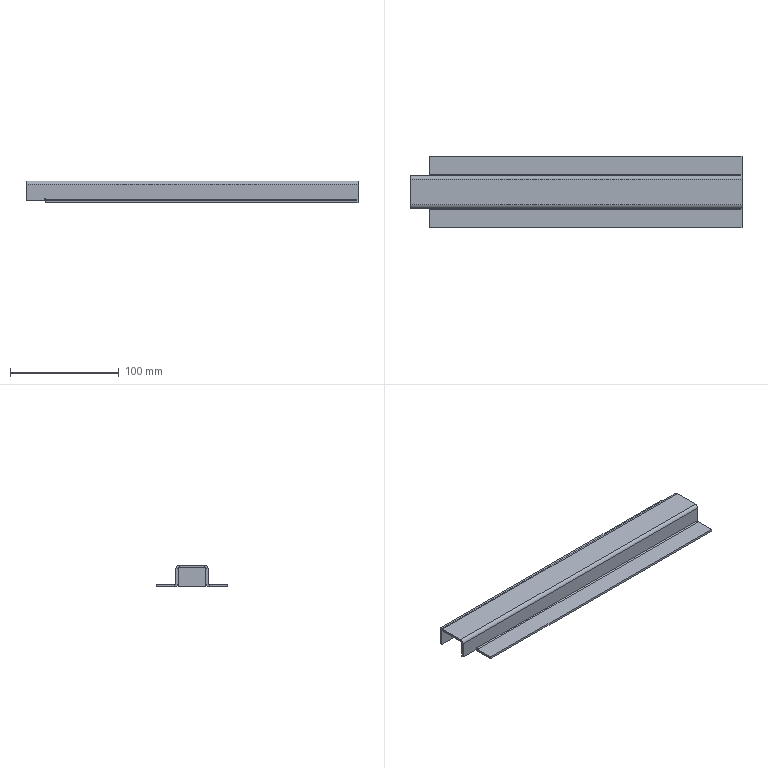Part | SolidWorks | features BaseBody 2 | 2 solids | 54 faces | box 304.9 x 65.5 x 20 mm | volume 59332 mm3 | plane 44 | cylinder 10 | commonest cylinder face diameters 2 x6 6 x4
STEP:
#1=CARTESIAN_POINT('',(-152.45,-14.75,-18.));
#2=VERTEX_POINT('',#1);
#3=CARTESIAN_POINT('',(-152.45,-12.75,-18.));
#4=VERTEX_POINT('',#3);
#5=CARTESIAN_POINT('',(-152.45,-32.75,-18.));
#6=DIRECTION('',(0.,1.,0.));
#7=VECTOR('',#6,1000.);
#8=LINE('',#5,#7);
#9=EDGE_CURVE('',#2,#4,#8,.T.);
#10=ORIENTED_EDGE('',*,*,#9,.T.);
#11=CARTESIAN_POINT('',(-135.45,-12.75,-18.));
#12=VERTEX_POINT('',#11);
#13=CARTESIAN_POINT('',(0.,-12.75,-18.));
#14=DIRECTION('',(1.,0.,0.));
#15=VECTOR('',#14,1000.);
#16=LINE('',#13,#15);
#17=EDGE_CURVE('',#4,#12,#16,.T.);
#18=ORIENTED_EDGE('',*,*,#17,.T.);
#19=CARTESIAN_POINT('',(-135.45,-14.75,-18.));
#20=VERTEX_POINT('',#19);
#21=CARTESIAN_POINT('',(-135.45,-32.75,-18.));
#22=DIRECTION('',(0.,1.,0.));
#23=VECTOR('',#22,1000.);
#24=LINE('',#21,#23);
#25=EDGE_CURVE('',#20,#12,#24,.T.);
#26=ORIENTED_EDGE('',*,*,#25,.F.);
#27=CARTESIAN_POINT('',(0.,-14.75,-18.));
#28=DIRECTION('',(1.,0.,0.));
#29=VECTOR('',#28,1000.);
#30=LINE('',#27,#29);
#31=EDGE_CURVE('',#2,#20,#30,.T.);
#32=ORIENTED_EDGE('',*,*,#31,.F.);
#33=EDGE_LOOP('',(#10,#18,#26,#32));
#34=FACE_OUTER_BOUND('',#33,.T.);
#35=CARTESIAN_POINT('',(-152.45,-32.75,-18.));
#36=DIRECTION('',(0.,0.,1.));
#37=DIRECTION('',(0.,-1.,0.));
#38=AXIS2_PLACEMENT_3D('',#35,#36,#37);
#39=PLANE('',#38);
#40=ADVANCED_FACE('',(#34),#39,.F.);
#41=CARTESIAN_POINT('',(-152.45,12.75,-18.));
#42=VERTEX_POINT('',#41);
#43=CARTESIAN_POINT('',(-152.45,14.75,-18.));
#44=VERTEX_POINT('',#43);
#45=CARTESIAN_POINT('',(-152.45,-32.75,-18.));
#46=DIRECTION('',(0.,1.,0.));
#47=VECTOR('',#46,1000.);
#48=LINE('',#45,#47);
#49=EDGE_CURVE('',#42,#44,#48,.T.);
#50=ORIENTED_EDGE('',*,*,#49,.T.);
#51=CARTESIAN_POINT('',(-135.45,14.75,-18.));
#52=VERTEX_POINT('',#51);
#53=CARTESIAN_POINT('',(-152.45,14.75,-18.));
#54=DIRECTION('',(1.,0.,0.));
#55=VECTOR('',#54,1000.);
#56=LINE('',#53,#55);
#57=EDGE_CURVE('',#44,#52,#56,.T.);
#58=ORIENTED_EDGE('',*,*,#57,.T.);
#59=CARTESIAN_POINT('',(-135.45,12.75,-18.));
#60=VERTEX_POINT('',#59);
#61=CARTESIAN_POINT('',(-135.45,14.75,-18.));
#62=DIRECTION('',(0.,-1.,0.));
#63=VECTOR('',#62,1000.);
#64=LINE('',#61,#63);
#65=EDGE_CURVE('',#52,#60,#64,.T.);
#66=ORIENTED_EDGE('',*,*,#65,.T.);
#67=CARTESIAN_POINT('',(0.,12.75,-18.));
#68=DIRECTION('',(1.,0.,0.));
#69=VECTOR('',#68,1000.);
#70=LINE('',#67,#69);
#71=EDGE_CURVE('',#42,#60,#70,.T.);
#72=ORIENTED_EDGE('',*,*,#71,.F.);
#73=EDGE_LOOP('',(#50,#58,#66,#72));
#74=FACE_OUTER_BOUND('',#73,.T.);
#75=CARTESIAN_POINT('',(-152.45,-32.75,-18.));
#76=DIRECTION('',(0.,0.,1.));
#77=DIRECTION('',(0.,-1.,0.));
#78=AXIS2_PLACEMENT_3D('',#75,#76,#77);
#79=PLANE('',#78);
#80=ADVANCED_FACE('',(#74),#79,.F.);
#81=CARTESIAN_POINT('',(-134.45,32.75,-18.));
#82=VERTEX_POINT('',#81);
#83=CARTESIAN_POINT('',(152.45,32.75,-18.));
#84=VERTEX_POINT('',#83);
#85=CARTESIAN_POINT('',(152.45,32.75,-18.));
#86=DIRECTION('',(1.,0.,0.));
#87=VECTOR('',#86,1000.);
#88=LINE('',#85,#87);
#89=EDGE_CURVE('',#82,#84,#88,.T.);
#90=ORIENTED_EDGE('',*,*,#89,.T.);
#91=CARTESIAN_POINT('',(152.45,32.75,-20.));
#92=VERTEX_POINT('',#91);
#93=CARTESIAN_POINT('',(152.45,32.75,-20.));
#94=DIRECTION('',(0.,0.,1.));
#95=VECTOR('',#94,1000.);
#96=LINE('',#93,#95);
#97=EDGE_CURVE('',#92,#84,#96,.T.);
#98=ORIENTED_EDGE('',*,*,#97,.F.);
#99=CARTESIAN_POINT('',(-134.45,32.75,-20.));
#100=VERTEX_POINT('',#99);
#101=CARTESIAN_POINT('',(0.,32.75,-20.));
#102=DIRECTION('',(1.,0.,0.));
#103=VECTOR('',#102,1000.);
#104=LINE('',#101,#103);
#105=EDGE_CURVE('',#100,#92,#104,.T.);
#106=ORIENTED_EDGE('',*,*,#105,.F.);
#107=CARTESIAN_POINT('',(-134.45,32.75,-20.));
#108=DIRECTION('',(0.,0.,1.));
#109=VECTOR('',#108,1000.);
#110=LINE('',#107,#109);
#111=EDGE_CURVE('',#100,#82,#110,.T.);
#112=ORIENTED_EDGE('',*,*,#111,.T.);
#113=EDGE_LOOP('',(#90,#98,#106,#112));
#114=FACE_OUTER_BOUND('',#113,.T.);
#115=CARTESIAN_POINT('',(152.45,32.75,-20.));
#116=DIRECTION('',(0.,-1.,0.));
#117=DIRECTION('',(-1.,0.,0.));
#118=AXIS2_PLACEMENT_3D('',#115,#116,#117);
#119=PLANE('',#118);
#120=ADVANCED_FACE('',(#114),#119,.F.);
#121=CARTESIAN_POINT('',(-134.45,15.75,-18.));
#122=VERTEX_POINT('',#121);
#123=CARTESIAN_POINT('',(-134.45,14.75,-18.));
#124=DIRECTION('',(0.,1.,0.));
#125=VECTOR('',#124,1000.);
#126=LINE('',#123,#125);
#127=EDGE_CURVE('',#122,#82,#126,.T.);
#128=ORIENTED_EDGE('',*,*,#127,.F.);
#129=CARTESIAN_POINT('',(152.45,15.75,-18.));
#130=VERTEX_POINT('',#129);
#131=CARTESIAN_POINT('',(152.45,15.75,-18.));
#132=DIRECTION('',(-1.,0.,0.));
#133=VECTOR('',#132,1000.);
#134=LINE('',#131,#133);
#135=EDGE_CURVE('',#130,#122,#134,.T.);
#136=ORIENTED_EDGE('',*,*,#135,.F.);
#137=CARTESIAN_POINT('',(152.45,14.75,-18.));
#138=DIRECTION('',(0.,-1.,0.));
#139=VECTOR('',#138,1000.);
#140=LINE('',#137,#139);
#141=EDGE_CURVE('',#84,#130,#140,.T.);
#142=ORIENTED_EDGE('',*,*,#141,.F.);
#143=ORIENTED_EDGE('',*,*,#89,.F.);
#144=EDGE_LOOP('',(#128,#136,#142,#143));
#145=FACE_OUTER_BOUND('',#144,.T.);
#146=CARTESIAN_POINT('',(0.,0.,-18.));
#147=DIRECTION('',(0.,0.,1.));
#148=DIRECTION('',(1.,0.,0.));
#149=AXIS2_PLACEMENT_3D('',#146,#147,#148);
#150=PLANE('',#149);
#151=ADVANCED_FACE('',(#145),#150,.T.);
#152=CARTESIAN_POINT('',(-134.45,15.75,-20.));
#153=VERTEX_POINT('',#152);
#154=CARTESIAN_POINT('',(152.45,15.75,-20.));
#155=VERTEX_POINT('',#154);
#156=CARTESIAN_POINT('',(152.45,15.75,-20.));
#157=DIRECTION('',(1.,0.,0.));
#158=VECTOR('',#157,1000.);
#159=LINE('',#156,#158);
#160=EDGE_CURVE('',#153,#155,#159,.T.);
#161=ORIENTED_EDGE('',*,*,#160,.F.);
#162=CARTESIAN_POINT('',(-134.45,0.,-20.));
#163=DIRECTION('',(0.,1.,0.));
#164=VECTOR('',#163,1000.);
#165=LINE('',#162,#164);
#166=EDGE_CURVE('',#153,#100,#165,.T.);
#167=ORIENTED_EDGE('',*,*,#166,.T.);
#168=ORIENTED_EDGE('',*,*,#105,.T.);
#169=CARTESIAN_POINT('',(152.45,0.,-20.));
#170=DIRECTION('',(0.,-1.,0.));
#171=VECTOR('',#170,1000.);
#172=LINE('',#169,#171);
#173=EDGE_CURVE('',#92,#155,#172,.T.);
#174=ORIENTED_EDGE('',*,*,#173,.T.);
#175=EDGE_LOOP('',(#161,#167,#168,#174));
#176=FACE_OUTER_BOUND('',#175,.T.);
#177=CARTESIAN_POINT('',(0.,0.,-20.));
#178=DIRECTION('',(0.,0.,1.));
#179=DIRECTION('',(1.,0.,0.));
#180=AXIS2_PLACEMENT_3D('',#177,#178,#179);
#181=PLANE('',#180);
#182=ADVANCED_FACE('',(#176),#181,.F.);
#183=CARTESIAN_POINT('',(-134.45,15.75,-18.));
#184=DIRECTION('',(0.,0.,-1.));
#185=VECTOR('',#184,1000.);
#186=LINE('',#183,#185);
#187=EDGE_CURVE('',#122,#153,#186,.T.);
#188=ORIENTED_EDGE('',*,*,#187,.F.);
#189=ORIENTED_EDGE('',*,*,#127,.T.);
#190=ORIENTED_EDGE('',*,*,#111,.F.);
#191=ORIENTED_EDGE('',*,*,#166,.F.);
#192=EDGE_LOOP('',(#188,#189,#190,#191));
#193=FACE_OUTER_BOUND('',#192,.T.);
#194=CARTESIAN_POINT('',(-134.45,14.75,-20.));
#195=DIRECTION('',(1.,0.,0.));
#196=DIRECTION('',(0.,1.,0.));
#197=AXIS2_PLACEMENT_3D('',#194,#195,#196);
#198=PLANE('',#197);
#199=ADVANCED_FACE('',(#193),#198,.F.);
#200=CARTESIAN_POINT('',(152.45,15.75,-20.));
#201=DIRECTION('',(0.,0.,-1.));
#202=VECTOR('',#201,1000.);
#203=LINE('',#200,#202);
#204=EDGE_CURVE('',#130,#155,#203,.T.);
#205=ORIENTED_EDGE('',*,*,#204,.T.);
#206=ORIENTED_EDGE('',*,*,#173,.F.);
#207=ORIENTED_EDGE('',*,*,#97,.T.);
#208=ORIENTED_EDGE('',*,*,#141,.T.);
#209=EDGE_LOOP('',(#205,#206,#207,#208));
#210=FACE_OUTER_BOUND('',#209,.T.);
#211=CARTESIAN_POINT('',(152.45,14.75,-20.));
#212=DIRECTION('',(-1.,0.,0.));
#213=DIRECTION('',(0.,0.,1.));
#214=AXIS2_PLACEMENT_3D('',#211,#212,#213);
#215=PLANE('',#214);
#216=ADVANCED_FACE('',(#210),#215,.F.);
#217=CARTESIAN_POINT('',(-134.45,14.75,-17.));
#218=VERTEX_POINT('',#217);
#219=CARTESIAN_POINT('',(152.45,14.75,-17.));
#220=VERTEX_POINT('',#219);
#221=CARTESIAN_POINT('',(-134.45,14.75,-17.));
#222=DIRECTION('',(1.,0.,0.));
#223=VECTOR('',#222,1000.);
#224=LINE('',#221,#223);
#225=EDGE_CURVE('',#218,#220,#224,.T.);
#226=ORIENTED_EDGE('',*,*,#225,.T.);
#227=CARTESIAN_POINT('',(152.45,15.75,-17.));
#228=DIRECTION('',(1.,0.,0.));
#229=DIRECTION('',(0.,0.,1.));
#230=AXIS2_PLACEMENT_3D('',#227,#228,#229);
#231=CIRCLE('',#230,1.);
#232=EDGE_CURVE('',#220,#130,#231,.T.);
#233=ORIENTED_EDGE('',*,*,#232,.T.);
#234=ORIENTED_EDGE('',*,*,#135,.T.);
#235=CARTESIAN_POINT('',(-134.45,15.75,-17.));
#236=DIRECTION('',(-1.,0.,0.));
#237=DIRECTION('',(0.,0.,1.));
#238=AXIS2_PLACEMENT_3D('',#235,#236,#237);
#239=CIRCLE('',#238,1.);
#240=EDGE_CURVE('',#122,#218,#239,.T.);
#241=ORIENTED_EDGE('',*,*,#240,.T.);
#242=EDGE_LOOP('',(#226,#233,#234,#241));
#243=FACE_OUTER_BOUND('',#242,.T.);
#244=CARTESIAN_POINT('',(-134.45,15.75,-17.));
#245=DIRECTION('',(-1.,0.,0.));
#246=DIRECTION('',(0.,0.,-1.));
#247=AXIS2_PLACEMENT_3D('',#244,#245,#246);
#248=CYLINDRICAL_SURFACE('',#247,1.);
#249=ADVANCED_FACE('',(#243),#248,.F.);
#250=CARTESIAN_POINT('',(-134.45,12.75,-17.));
#251=VERTEX_POINT('',#250);
#252=CARTESIAN_POINT('',(152.45,12.75,-17.));
#253=VERTEX_POINT('',#252);
#254=CARTESIAN_POINT('',(-134.45,12.75,-17.));
#255=DIRECTION('',(1.,0.,0.));
#256=VECTOR('',#255,1000.);
#257=LINE('',#254,#256);
#258=EDGE_CURVE('',#251,#253,#257,.T.);
#259=ORIENTED_EDGE('',*,*,#258,.F.);
#260=CARTESIAN_POINT('',(-134.45,15.75,-17.));
#261=DIRECTION('',(-1.,0.,0.));
#262=DIRECTION('',(0.,0.,1.));
#263=AXIS2_PLACEMENT_3D('',#260,#261,#262);
#264=CIRCLE('',#263,3.);
#265=EDGE_CURVE('',#153,#251,#264,.T.);
#266=ORIENTED_EDGE('',*,*,#265,.F.);
#267=ORIENTED_EDGE('',*,*,#160,.T.);
#268=CARTESIAN_POINT('',(152.45,15.75,-17.));
#269=DIRECTION('',(1.,0.,0.));
#270=DIRECTION('',(0.,0.,1.));
#271=AXIS2_PLACEMENT_3D('',#268,#269,#270);
#272=CIRCLE('',#271,3.);
#273=EDGE_CURVE('',#253,#155,#272,.T.);
#274=ORIENTED_EDGE('',*,*,#273,.F.);
#275=EDGE_LOOP('',(#259,#266,#267,#274));
#276=FACE_OUTER_BOUND('',#275,.T.);
#277=CARTESIAN_POINT('',(-134.45,15.75,-17.));
#278=DIRECTION('',(-1.,0.,0.));
#279=DIRECTION('',(0.,0.,-1.));
#280=AXIS2_PLACEMENT_3D('',#277,#278,#279);
#281=CYLINDRICAL_SURFACE('',#280,3.);
#282=ADVANCED_FACE('',(#276),#281,.T.);
#283=ORIENTED_EDGE('',*,*,#240,.F.);
#284=ORIENTED_EDGE('',*,*,#187,.T.);
#285=ORIENTED_EDGE('',*,*,#265,.T.);
#286=CARTESIAN_POINT('',(-134.45,14.75,-17.));
#287=DIRECTION('',(0.,-1.,0.));
#288=VECTOR('',#287,1000.);
#289=LINE('',#286,#288);
#290=EDGE_CURVE('',#218,#251,#289,.T.);
#291=ORIENTED_EDGE('',*,*,#290,.F.);
#292=EDGE_LOOP('',(#283,#284,#285,#291));
#293=FACE_OUTER_BOUND('',#292,.T.);
#294=CARTESIAN_POINT('',(-134.45,15.75,-17.));
#295=DIRECTION('',(1.,0.,0.));
#296=DIRECTION('',(0.,1.,0.));
#297=AXIS2_PLACEMENT_3D('',#294,#295,#296);
#298=PLANE('',#297);
#299=ADVANCED_FACE('',(#293),#298,.F.);
#300=ORIENTED_EDGE('',*,*,#204,.F.);
#301=ORIENTED_EDGE('',*,*,#232,.F.);
#302=CARTESIAN_POINT('',(152.45,14.75,-17.));
#303=DIRECTION('',(0.,-1.,0.));
#304=VECTOR('',#303,1000.);
#305=LINE('',#302,#304);
#306=EDGE_CURVE('',#220,#253,#305,.T.);
#307=ORIENTED_EDGE('',*,*,#306,.T.);
#308=ORIENTED_EDGE('',*,*,#273,.T.);
#309=EDGE_LOOP('',(#300,#301,#307,#308));
#310=FACE_OUTER_BOUND('',#309,.T.);
#311=CARTESIAN_POINT('',(152.45,15.75,-17.));
#312=DIRECTION('',(1.,0.,0.));
#313=DIRECTION('',(0.,1.,0.));
#314=AXIS2_PLACEMENT_3D('',#311,#312,#313);
#315=PLANE('',#314);
#316=ADVANCED_FACE('',(#310),#315,.T.);
#317=ORIENTED_EDGE('',*,*,#65,.F.);
#318=CARTESIAN_POINT('',(-135.45,14.75,-16.));
#319=VERTEX_POINT('',#318);
#320=CARTESIAN_POINT('',(-135.45,14.75,-20.));
#321=DIRECTION('',(0.,0.,1.));
#322=VECTOR('',#321,1000.);
#323=LINE('',#320,#322);
#324=EDGE_CURVE('',#52,#319,#323,.T.);
#325=ORIENTED_EDGE('',*,*,#324,.T.);
#326=CARTESIAN_POINT('',(-135.45,12.75,-16.));
#327=VERTEX_POINT('',#326);
#328=CARTESIAN_POINT('',(-135.45,14.75,-16.));
#329=DIRECTION('',(0.,-1.,0.));
#330=VECTOR('',#329,1000.);
#331=LINE('',#328,#330);
#332=EDGE_CURVE('',#319,#327,#331,.T.);
#333=ORIENTED_EDGE('',*,*,#332,.T.);
#334=CARTESIAN_POINT('',(-135.45,12.75,0.));
#335=DIRECTION('',(0.,0.,-1.));
#336=VECTOR('',#335,1000.);
#337=LINE('',#334,#336);
#338=EDGE_CURVE('',#327,#60,#337,.T.);
#339=ORIENTED_EDGE('',*,*,#338,.T.);
#340=EDGE_LOOP('',(#317,#325,#333,#339));
#341=FACE_OUTER_BOUND('',#340,.T.);
#342=CARTESIAN_POINT('',(-135.45,14.75,-20.));
#343=DIRECTION('',(1.,0.,0.));
#344=DIRECTION('',(0.,1.,0.));
#345=AXIS2_PLACEMENT_3D('',#342,#343,#344);
#346=PLANE('',#345);
#347=ADVANCED_FACE('',(#341),#346,.T.);
#348=ORIENTED_EDGE('',*,*,#290,.T.);
#349=CARTESIAN_POINT('',(-134.45,12.75,-16.));
#350=VERTEX_POINT('',#349);
#351=CARTESIAN_POINT('',(-134.45,12.75,0.));
#352=DIRECTION('',(0.,0.,1.));
#353=VECTOR('',#352,1000.);
#354=LINE('',#351,#353);
#355=EDGE_CURVE('',#251,#350,#354,.T.);
#356=ORIENTED_EDGE('',*,*,#355,.T.);
#357=CARTESIAN_POINT('',(-134.45,14.75,-16.));
#358=VERTEX_POINT('',#357);
#359=CARTESIAN_POINT('',(-134.45,14.75,-16.));
#360=DIRECTION('',(0.,-1.,0.));
#361=VECTOR('',#360,1000.);
#362=LINE('',#359,#361);
#363=EDGE_CURVE('',#358,#350,#362,.T.);
#364=ORIENTED_EDGE('',*,*,#363,.F.);
#365=CARTESIAN_POINT('',(-134.45,14.75,-16.));
#366=DIRECTION('',(0.,0.,-1.));
#367=VECTOR('',#366,1000.);
#368=LINE('',#365,#367);
#369=EDGE_CURVE('',#358,#218,#368,.T.);
#370=ORIENTED_EDGE('',*,*,#369,.T.);
#371=EDGE_LOOP('',(#348,#356,#364,#370));
#372=FACE_OUTER_BOUND('',#371,.T.);
#373=CARTESIAN_POINT('',(-134.45,14.75,-16.));
#374=DIRECTION('',(-1.,0.,0.));
#375=DIRECTION('',(0.,0.,1.));
#376=AXIS2_PLACEMENT_3D('',#373,#374,#375);
#377=PLANE('',#376);
#378=ADVANCED_FACE('',(#372),#377,.T.);
#379=ORIENTED_EDGE('',*,*,#363,.T.);
#380=CARTESIAN_POINT('',(0.,12.75,-16.));
#381=DIRECTION('',(-1.,0.,0.));
#382=VECTOR('',#381,1000.);
#383=LINE('',#380,#382);
#384=EDGE_CURVE('',#350,#327,#383,.T.);
#385=ORIENTED_EDGE('',*,*,#384,.T.);
#386=ORIENTED_EDGE('',*,*,#332,.F.);
#387=CARTESIAN_POINT('',(-135.45,14.75,-16.));
#388=DIRECTION('',(1.,0.,0.));
#389=VECTOR('',#388,1000.);
#390=LINE('',#387,#389);
#391=EDGE_CURVE('',#319,#358,#390,.T.);
#392=ORIENTED_EDGE('',*,*,#391,.T.);
#393=EDGE_LOOP('',(#379,#385,#386,#392));
#394=FACE_OUTER_BOUND('',#393,.T.);
#395=CARTESIAN_POINT('',(-135.45,14.75,-16.));
#396=DIRECTION('',(0.,0.,-1.));
#397=DIRECTION('',(-1.,0.,0.));
#398=AXIS2_PLACEMENT_3D('',#395,#396,#397);
#399=PLANE('',#398);
#400=ADVANCED_FACE('',(#394),#399,.T.);
#401=CARTESIAN_POINT('',(-134.45,-32.75,-18.));
#402=VERTEX_POINT('',#401);
#403=CARTESIAN_POINT('',(152.45,-32.75,-18.));
#404=VERTEX_POINT('',#403);
#405=CARTESIAN_POINT('',(0.,-32.75,-18.));
#406=DIRECTION('',(1.,0.,0.));
#407=VECTOR('',#406,1000.);
#408=LINE('',#405,#407);
#409=EDGE_CURVE('',#402,#404,#408,.T.);
#410=ORIENTED_EDGE('',*,*,#409,.F.);
#411=CARTESIAN_POINT('',(-134.45,-32.75,-20.));
#412=VERTEX_POINT('',#411);
#413=CARTESIAN_POINT('',(-134.45,-32.75,-20.));
#414=DIRECTION('',(0.,0.,1.));
#415=VECTOR('',#414,1000.);
#416=LINE('',#413,#415);
#417=EDGE_CURVE('',#412,#402,#416,.T.);
#418=ORIENTED_EDGE('',*,*,#417,.F.);
#419=CARTESIAN_POINT('',(152.45,-32.75,-20.));
#420=VERTEX_POINT('',#419);
#421=CARTESIAN_POINT('',(-134.45,-32.75,-20.));
#422=DIRECTION('',(1.,0.,0.));
#423=VECTOR('',#422,1000.);
#424=LINE('',#421,#423);
#425=EDGE_CURVE('',#412,#420,#424,.T.);
#426=ORIENTED_EDGE('',*,*,#425,.T.);
#427=CARTESIAN_POINT('',(152.45,-32.75,-20.));
#428=DIRECTION('',(0.,0.,1.));
#429=VECTOR('',#428,1000.);
#430=LINE('',#427,#429);
#431=EDGE_CURVE('',#420,#404,#430,.T.);
#432=ORIENTED_EDGE('',*,*,#431,.T.);
#433=EDGE_LOOP('',(#410,#418,#426,#432));
#434=FACE_OUTER_BOUND('',#433,.T.);
#435=CARTESIAN_POINT('',(-134.45,-32.75,-20.));
#436=DIRECTION('',(0.,-1.,0.));
#437=DIRECTION('',(0.,0.,-1.));
#438=AXIS2_PLACEMENT_3D('',#435,#436,#437);
#439=PLANE('',#438);
#440=ADVANCED_FACE('',(#434),#439,.T.);
#441=CARTESIAN_POINT('',(-134.45,-15.75,-18.));
#442=VERTEX_POINT('',#441);
#443=CARTESIAN_POINT('',(152.45,-15.75,-18.));
#444=VERTEX_POINT('',#443);
#445=CARTESIAN_POINT('',(-134.45,-15.75,-18.));
#446=DIRECTION('',(1.,0.,0.));
#447=VECTOR('',#446,1000.);
#448=LINE('',#445,#447);
#449=EDGE_CURVE('',#442,#444,#448,.T.);
#450=ORIENTED_EDGE('',*,*,#449,.F.);
#451=CARTESIAN_POINT('',(-134.45,0.,-18.));
#452=DIRECTION('',(0.,-1.,0.));
#453=VECTOR('',#452,1000.);
#454=LINE('',#451,#453);
#455=EDGE_CURVE('',#442,#402,#454,.T.);
#456=ORIENTED_EDGE('',*,*,#455,.T.);
#457=ORIENTED_EDGE('',*,*,#409,.T.);
#458=CARTESIAN_POINT('',(152.45,0.,-18.));
#459=DIRECTION('',(0.,1.,0.));
#460=VECTOR('',#459,1000.);
#461=LINE('',#458,#460);
#462=EDGE_CURVE('',#404,#444,#461,.T.);
#463=ORIENTED_EDGE('',*,*,#462,.T.);
#464=EDGE_LOOP('',(#450,#456,#457,#463));
#465=FACE_OUTER_BOUND('',#464,.T.);
#466=CARTESIAN_POINT('',(0.,0.,-18.));
#467=DIRECTION('',(0.,0.,-1.));
#468=DIRECTION('',(-1.,0.,0.));
#469=AXIS2_PLACEMENT_3D('',#466,#467,#468);
#470=PLANE('',#469);
#471=ADVANCED_FACE('',(#465),#470,.F.);
#472=CARTESIAN_POINT('',(-134.45,-15.75,-20.));
#473=VERTEX_POINT('',#472);
#474=CARTESIAN_POINT('',(-134.45,-14.75,-20.));
#475=DIRECTION('',(0.,-1.,0.));
#476=VECTOR('',#475,1000.);
#477=LINE('',#474,#476);
#478=EDGE_CURVE('',#473,#412,#477,.T.);
#479=ORIENTED_EDGE('',*,*,#478,.F.);
#480=CARTESIAN_POINT('',(152.45,-15.75,-20.));
#481=VERTEX_POINT('',#480);
#482=CARTESIAN_POINT('',(0.,-15.75,-20.));
#483=DIRECTION('',(1.,0.,0.));
#484=VECTOR('',#483,1000.);
#485=LINE('',#482,#484);
#486=EDGE_CURVE('',#473,#481,#485,.T.);
#487=ORIENTED_EDGE('',*,*,#486,.T.);
#488=CARTESIAN_POINT('',(152.45,-32.75,-20.));
#489=DIRECTION('',(0.,1.,0.));
#490=VECTOR('',#489,1000.);
#491=LINE('',#488,#490);
#492=EDGE_CURVE('',#420,#481,#491,.T.);
#493=ORIENTED_EDGE('',*,*,#492,.F.);
#494=ORIENTED_EDGE('',*,*,#425,.F.);
#495=EDGE_LOOP('',(#479,#487,#493,#494));
#496=FACE_OUTER_BOUND('',#495,.T.);
#497=CARTESIAN_POINT('',(0.,0.,-20.));
#498=DIRECTION('',(0.,0.,-1.));
#499=DIRECTION('',(-1.,0.,0.));
#500=AXIS2_PLACEMENT_3D('',#497,#498,#499);
#501=PLANE('',#500);
#502=ADVANCED_FACE('',(#496),#501,.T.);
#503=ORIENTED_EDGE('',*,*,#455,.F.);
#504=CARTESIAN_POINT('',(-134.45,-15.75,-20.));
#505=DIRECTION('',(0.,0.,-1.));
#506=VECTOR('',#505,1000.);
#507=LINE('',#504,#506);
#508=EDGE_CURVE('',#442,#473,#507,.T.);
#509=ORIENTED_EDGE('',*,*,#508,.T.);
#510=ORIENTED_EDGE('',*,*,#478,.T.);
#511=ORIENTED_EDGE('',*,*,#417,.T.);
#512=EDGE_LOOP('',(#503,#509,#510,#511));
#513=FACE_OUTER_BOUND('',#512,.T.);
#514=CARTESIAN_POINT('',(-134.45,-14.75,-20.));
#515=DIRECTION('',(-1.,0.,0.));
#516=DIRECTION('',(0.,1.,0.));
#517=AXIS2_PLACEMENT_3D('',#514,#515,#516);
#518=PLANE('',#517);
#519=ADVANCED_FACE('',(#513),#518,.T.);
#520=ORIENTED_EDGE('',*,*,#492,.T.);
#521=CARTESIAN_POINT('',(152.45,-15.75,-18.));
#522=DIRECTION('',(0.,0.,-1.));
#523=VECTOR('',#522,1000.);
#524=LINE('',#521,#523);
#525=EDGE_CURVE('',#444,#481,#524,.T.);
#526=ORIENTED_EDGE('',*,*,#525,.F.);
#527=ORIENTED_EDGE('',*,*,#462,.F.);
#528=ORIENTED_EDGE('',*,*,#431,.F.);
#529=EDGE_LOOP('',(#520,#526,#527,#528));
#530=FACE_OUTER_BOUND('',#529,.T.);
#531=CARTESIAN_POINT('',(152.45,-32.75,-20.));
#532=DIRECTION('',(1.,0.,0.));
#533=DIRECTION('',(0.,0.,-1.));
#534=AXIS2_PLACEMENT_3D('',#531,#532,#533);
#535=PLANE('',#534);
#536=ADVANCED_FACE('',(#530),#535,.T.);
#537=CARTESIAN_POINT('',(152.45,-14.75,-17.));
#538=VERTEX_POINT('',#537);
#539=CARTESIAN_POINT('',(-134.45,-14.75,-17.));
#540=VERTEX_POINT('',#539);
#541=CARTESIAN_POINT('',(152.45,-14.75,-17.));
#542=DIRECTION('',(-1.,0.,0.));
#543=VECTOR('',#542,1000.);
#544=LINE('',#541,#543);
#545=EDGE_CURVE('',#538,#540,#544,.T.);
#546=ORIENTED_EDGE('',*,*,#545,.T.);
#547=CARTESIAN_POINT('',(-134.45,-15.75,-17.));
#548=DIRECTION('',(-1.,0.,0.));
#549=DIRECTION('',(0.,0.,-1.));
#550=AXIS2_PLACEMENT_3D('',#547,#548,#549);
#551=CIRCLE('',#550,1.);
#552=EDGE_CURVE('',#540,#442,#551,.T.);
#553=ORIENTED_EDGE('',*,*,#552,.T.);
#554=ORIENTED_EDGE('',*,*,#449,.T.);
#555=CARTESIAN_POINT('',(152.45,-15.75,-17.));
#556=DIRECTION('',(1.,0.,0.));
#557=DIRECTION('',(0.,0.,-1.));
#558=AXIS2_PLACEMENT_3D('',#555,#556,#557);
#559=CIRCLE('',#558,1.);
#560=EDGE_CURVE('',#444,#538,#559,.T.);
#561=ORIENTED_EDGE('',*,*,#560,.T.);
#562=EDGE_LOOP('',(#546,#553,#554,#561));
#563=FACE_OUTER_BOUND('',#562,.T.);
#564=CARTESIAN_POINT('',(152.45,-15.75,-17.));
#565=DIRECTION('',(1.,0.,0.));
#566=DIRECTION('',(0.,0.,-1.));
#567=AXIS2_PLACEMENT_3D('',#564,#565,#566);
#568=CYLINDRICAL_SURFACE('',#567,1.);
#569=ADVANCED_FACE('',(#563),#568,.F.);
#570=CARTESIAN_POINT('',(152.45,-12.75,-17.));
#571=VERTEX_POINT('',#570);
#572=CARTESIAN_POINT('',(-134.45,-12.75,-17.));
#573=VERTEX_POINT('',#572);
#574=CARTESIAN_POINT('',(152.45,-12.75,-17.));
#575=DIRECTION('',(-1.,0.,0.));
#576=VECTOR('',#575,1000.);
#577=LINE('',#574,#576);
#578=EDGE_CURVE('',#571,#573,#577,.T.);
#579=ORIENTED_EDGE('',*,*,#578,.F.);
#580=CARTESIAN_POINT('',(152.45,-15.75,-17.));
#581=DIRECTION('',(1.,0.,0.));
#582=DIRECTION('',(0.,0.,-1.));
#583=AXIS2_PLACEMENT_3D('',#580,#581,#582);
#584=CIRCLE('',#583,3.);
#585=EDGE_CURVE('',#481,#571,#584,.T.);
#586=ORIENTED_EDGE('',*,*,#585,.F.);
#587=ORIENTED_EDGE('',*,*,#486,.F.);
#588=CARTESIAN_POINT('',(-134.45,-15.75,-17.));
#589=DIRECTION('',(-1.,0.,0.));
#590=DIRECTION('',(0.,0.,-1.));
#591=AXIS2_PLACEMENT_3D('',#588,#589,#590);
#592=CIRCLE('',#591,3.);
#593=EDGE_CURVE('',#573,#473,#592,.T.);
#594=ORIENTED_EDGE('',*,*,#593,.F.);
#595=EDGE_LOOP('',(#579,#586,#587,#594));
#596=FACE_OUTER_BOUND('',#595,.T.);
#597=CARTESIAN_POINT('',(152.45,-15.75,-17.));
#598=DIRECTION('',(1.,0.,0.));
#599=DIRECTION('',(0.,0.,-1.));
#600=AXIS2_PLACEMENT_3D('',#597,#598,#599);
#601=CYLINDRICAL_SURFACE('',#600,3.);
#602=ADVANCED_FACE('',(#596),#601,.T.);
#603=ORIENTED_EDGE('',*,*,#560,.F.);
#604=ORIENTED_EDGE('',*,*,#525,.T.);
#605=ORIENTED_EDGE('',*,*,#585,.T.);
#606=CARTESIAN_POINT('',(152.45,-14.75,-17.));
#607=DIRECTION('',(0.,1.,0.));
#608=VECTOR('',#607,1000.);
#609=LINE('',#606,#608);
#610=EDGE_CURVE('',#538,#571,#609,.T.);
#611=ORIENTED_EDGE('',*,*,#610,.F.);
#612=EDGE_LOOP('',(#603,#604,#605,#611));
#613=FACE_OUTER_BOUND('',#612,.T.);
#614=CARTESIAN_POINT('',(152.45,-15.75,-17.));
#615=DIRECTION('',(-1.,0.,0.));
#616=DIRECTION('',(0.,0.,1.));
#617=AXIS2_PLACEMENT_3D('',#614,#615,#616);
#618=PLANE('',#617);
#619=ADVANCED_FACE('',(#613),#618,.F.);
#620=ORIENTED_EDGE('',*,*,#508,.F.);
#621=ORIENTED_EDGE('',*,*,#552,.F.);
#622=CARTESIAN_POINT('',(-134.45,-14.75,-17.));
#623=DIRECTION('',(0.,1.,0.));
#624=VECTOR('',#623,1000.);
#625=LINE('',#622,#624);
#626=EDGE_CURVE('',#540,#573,#625,.T.);
#627=ORIENTED_EDGE('',*,*,#626,.T.);
#628=ORIENTED_EDGE('',*,*,#593,.T.);
#629=EDGE_LOOP('',(#620,#621,#627,#628));
#630=FACE_OUTER_BOUND('',#629,.T.);
#631=CARTESIAN_POINT('',(-134.45,-15.75,-17.));
#632=DIRECTION('',(-1.,0.,0.));
#633=DIRECTION('',(0.,0.,1.));
#634=AXIS2_PLACEMENT_3D('',#631,#632,#633);
#635=PLANE('',#634);
#636=ADVANCED_FACE('',(#630),#635,.T.);
#637=ORIENTED_EDGE('',*,*,#25,.T.);
#638=CARTESIAN_POINT('',(-135.45,-12.75,-16.));
#639=VERTEX_POINT('',#638);
#640=CARTESIAN_POINT('',(-135.45,-12.75,0.));
#641=DIRECTION('',(0.,0.,-1.));
#642=VECTOR('',#641,1000.);
#643=LINE('',#640,#642);
#644=EDGE_CURVE('',#639,#12,#643,.T.);
#645=ORIENTED_EDGE('',*,*,#644,.F.);
#646=CARTESIAN_POINT('',(-135.45,-14.75,-16.));
#647=VERTEX_POINT('',#646);
#648=CARTESIAN_POINT('',(-135.45,-14.75,-16.));
#649=DIRECTION('',(0.,1.,0.));
#650=VECTOR('',#649,1000.);
#651=LINE('',#648,#650);
#652=EDGE_CURVE('',#647,#639,#651,.T.);
#653=ORIENTED_EDGE('',*,*,#652,.F.);
#654=CARTESIAN_POINT('',(-135.45,-14.75,-16.));
#655=DIRECTION('',(0.,0.,-1.));
#656=VECTOR('',#655,1000.);
#657=LINE('',#654,#656);
#658=EDGE_CURVE('',#647,#20,#657,.T.);
#659=ORIENTED_EDGE('',*,*,#658,.T.);
#660=EDGE_LOOP('',(#637,#645,#653,#659));
#661=FACE_OUTER_BOUND('',#660,.T.);
#662=CARTESIAN_POINT('',(-135.45,-14.75,-16.));
#663=DIRECTION('',(1.,0.,0.));
#664=DIRECTION('',(0.,0.,-1.));
#665=AXIS2_PLACEMENT_3D('',#662,#663,#664);
#666=PLANE('',#665);
#667=ADVANCED_FACE('',(#661),#666,.T.);
#668=CARTESIAN_POINT('',(-134.45,-12.75,-16.));
#669=VERTEX_POINT('',#668);
#670=CARTESIAN_POINT('',(0.,-12.75,-16.));
#671=DIRECTION('',(-1.,0.,0.));
#672=VECTOR('',#671,1000.);
#673=LINE('',#670,#672);
#674=EDGE_CURVE('',#669,#639,#673,.T.);
#675=ORIENTED_EDGE('',*,*,#674,.F.);
#676=CARTESIAN_POINT('',(-134.45,-14.75,-16.));
#677=VERTEX_POINT('',#676);
#678=CARTESIAN_POINT('',(-134.45,-14.75,-16.));
#679=DIRECTION('',(0.,1.,0.));
#680=VECTOR('',#679,1000.);
#681=LINE('',#678,#680);
#682=EDGE_CURVE('',#677,#669,#681,.T.);
#683=ORIENTED_EDGE('',*,*,#682,.F.);
#684=CARTESIAN_POINT('',(-134.45,-14.75,-16.));
#685=DIRECTION('',(-1.,0.,0.));
#686=VECTOR('',#685,1000.);
#687=LINE('',#684,#686);
#688=EDGE_CURVE('',#677,#647,#687,.T.);
#689=ORIENTED_EDGE('',*,*,#688,.T.);
#690=ORIENTED_EDGE('',*,*,#652,.T.);
#691=EDGE_LOOP('',(#675,#683,#689,#690));
#692=FACE_OUTER_BOUND('',#691,.T.);
#693=CARTESIAN_POINT('',(-134.45,-14.75,-16.));
#694=DIRECTION('',(0.,0.,-1.));
#695=DIRECTION('',(0.,-1.,0.));
#696=AXIS2_PLACEMENT_3D('',#693,#694,#695);
#697=PLANE('',#696);
#698=ADVANCED_FACE('',(#692),#697,.T.);
#699=CARTESIAN_POINT('',(-134.45,-12.75,0.));
#700=DIRECTION('',(0.,0.,1.));
#701=VECTOR('',#700,1000.);
#702=LINE('',#699,#701);
#703=EDGE_CURVE('',#573,#669,#702,.T.);
#704=ORIENTED_EDGE('',*,*,#703,.F.);
#705=ORIENTED_EDGE('',*,*,#626,.F.);
#706=CARTESIAN_POINT('',(-134.45,-14.75,-17.));
#707=DIRECTION('',(0.,0.,1.));
#708=VECTOR('',#707,1000.);
#709=LINE('',#706,#708);
#710=EDGE_CURVE('',#540,#677,#709,.T.);
#711=ORIENTED_EDGE('',*,*,#710,.T.);
#712=ORIENTED_EDGE('',*,*,#682,.T.);
#713=EDGE_LOOP('',(#704,#705,#711,#712));
#714=FACE_OUTER_BOUND('',#713,.T.);
#715=CARTESIAN_POINT('',(-134.45,-14.75,-17.));
#716=DIRECTION('',(-1.,0.,0.));
#717=DIRECTION('',(0.,1.,0.));
#718=AXIS2_PLACEMENT_3D('',#715,#716,#717);
#719=PLANE('',#718);
#720=ADVANCED_FACE('',(#714),#719,.T.);
#721=ORIENTED_EDGE('',*,*,#9,.F.);
#722=CARTESIAN_POINT('',(-152.45,-14.75,-3.));
#723=VERTEX_POINT('',#722);
#724=CARTESIAN_POINT('',(-152.45,-14.75,-20.));
#725=DIRECTION('',(0.,0.,1.));
#726=VECTOR('',#725,1000.);
#727=LINE('',#724,#726);
#728=EDGE_CURVE('',#2,#723,#727,.T.);
#729=ORIENTED_EDGE('',*,*,#728,.T.);
#730=CARTESIAN_POINT('',(-152.45,-12.75,-3.));
#731=VERTEX_POINT('',#730);
#732=CARTESIAN_POINT('',(-152.45,-12.75,-3.));
#733=DIRECTION('',(0.,-1.,0.));
#734=VECTOR('',#733,1000.);
#735=LINE('',#732,#734);
#736=EDGE_CURVE('',#731,#723,#735,.T.);
#737=ORIENTED_EDGE('',*,*,#736,.F.);
#738=CARTESIAN_POINT('',(-152.45,-12.75,0.));
#739=DIRECTION('',(0.,0.,1.));
#740=VECTOR('',#739,1000.);
#741=LINE('',#738,#740);
#742=EDGE_CURVE('',#4,#731,#741,.T.);
#743=ORIENTED_EDGE('',*,*,#742,.F.);
#744=EDGE_LOOP('',(#721,#729,#737,#743));
#745=FACE_OUTER_BOUND('',#744,.T.);
#746=CARTESIAN_POINT('',(-152.45,-14.75,-20.));
#747=DIRECTION('',(-1.,0.,0.));
#748=DIRECTION('',(0.,0.,1.));
#749=AXIS2_PLACEMENT_3D('',#746,#747,#748);
#750=PLANE('',#749);
#751=ADVANCED_FACE('',(#745),#750,.T.);
#752=CARTESIAN_POINT('',(-152.45,-11.75,-2.));
#753=VERTEX_POINT('',#752);
#754=CARTESIAN_POINT('',(152.45,-11.75,-2.));
#755=VERTEX_POINT('',#754);
#756=CARTESIAN_POINT('',(-152.45,-11.75,-2.));
#757=DIRECTION('',(1.,0.,0.));
#758=VECTOR('',#757,1000.);
#759=LINE('',#756,#758);
#760=EDGE_CURVE('',#753,#755,#759,.T.);
#761=ORIENTED_EDGE('',*,*,#760,.T.);
#762=CARTESIAN_POINT('',(152.45,-12.75,-3.));
#763=VERTEX_POINT('',#762);
#764=CARTESIAN_POINT('',(152.45,-11.75,-3.));
#765=DIRECTION('',(1.,0.,0.));
#766=DIRECTION('',(0.,0.,1.));
#767=AXIS2_PLACEMENT_3D('',#764,#765,#766);
#768=CIRCLE('',#767,1.);
#769=EDGE_CURVE('',#755,#763,#768,.T.);
#770=ORIENTED_EDGE('',*,*,#769,.T.);
#771=CARTESIAN_POINT('',(152.45,-12.75,-3.));
#772=DIRECTION('',(-1.,0.,0.));
#773=VECTOR('',#772,1000.);
#774=LINE('',#771,#773);
#775=EDGE_CURVE('',#763,#731,#774,.T.);
#776=ORIENTED_EDGE('',*,*,#775,.T.);
#777=CARTESIAN_POINT('',(-152.45,-11.75,-3.));
#778=DIRECTION('',(-1.,0.,0.));
#779=DIRECTION('',(0.,0.,1.));
#780=AXIS2_PLACEMENT_3D('',#777,#778,#779);
#781=CIRCLE('',#780,1.);
#782=EDGE_CURVE('',#731,#753,#781,.T.);
#783=ORIENTED_EDGE('',*,*,#782,.T.);
#784=EDGE_LOOP('',(#761,#770,#776,#783));
#785=FACE_OUTER_BOUND('',#784,.T.);
#786=CARTESIAN_POINT('',(-152.45,-11.75,-3.));
#787=DIRECTION('',(-1.,0.,0.));
#788=DIRECTION('',(0.,-1.,0.));
#789=AXIS2_PLACEMENT_3D('',#786,#787,#788);
#790=CYLINDRICAL_SURFACE('',#789,1.);
#791=ADVANCED_FACE('',(#785),#790,.F.);
#792=CARTESIAN_POINT('',(-152.45,-11.75,0.));
#793=VERTEX_POINT('',#792);
#794=CARTESIAN_POINT('',(152.45,-11.75,0.));
#795=VERTEX_POINT('',#794);
#796=CARTESIAN_POINT('',(-152.45,-11.75,0.));
#797=DIRECTION('',(1.,0.,0.));
#798=VECTOR('',#797,1000.);
#799=LINE('',#796,#798);
#800=EDGE_CURVE('',#793,#795,#799,.T.);
#801=ORIENTED_EDGE('',*,*,#800,.F.);
#802=CARTESIAN_POINT('',(-152.45,-11.75,-3.));
#803=DIRECTION('',(-1.,0.,0.));
#804=DIRECTION('',(0.,0.,1.));
#805=AXIS2_PLACEMENT_3D('',#802,#803,#804);
#806=CIRCLE('',#805,3.);
#807=EDGE_CURVE('',#723,#793,#806,.T.);
#808=ORIENTED_EDGE('',*,*,#807,.F.);
#809=CARTESIAN_POINT('',(152.45,-14.75,-3.));
#810=VERTEX_POINT('',#809);
#811=CARTESIAN_POINT('',(152.45,-14.75,-3.));
#812=DIRECTION('',(1.,0.,0.));
#813=VECTOR('',#812,1000.);
#814=LINE('',#811,#813);
#815=EDGE_CURVE('',#723,#810,#814,.T.);
#816=ORIENTED_EDGE('',*,*,#815,.T.);
#817=CARTESIAN_POINT('',(152.45,-11.75,-3.));
#818=DIRECTION('',(1.,0.,0.));
#819=DIRECTION('',(0.,0.,1.));
#820=AXIS2_PLACEMENT_3D('',#817,#818,#819);
#821=CIRCLE('',#820,3.);
#822=EDGE_CURVE('',#795,#810,#821,.T.);
#823=ORIENTED_EDGE('',*,*,#822,.F.);
#824=EDGE_LOOP('',(#801,#808,#816,#823));
#825=FACE_OUTER_BOUND('',#824,.T.);
#826=CARTESIAN_POINT('',(-152.45,-11.75,-3.));
#827=DIRECTION('',(-1.,0.,0.));
#828=DIRECTION('',(0.,-1.,0.));
#829=AXIS2_PLACEMENT_3D('',#826,#827,#828);
#830=CYLINDRICAL_SURFACE('',#829,3.);
#831=ADVANCED_FACE('',(#825),#830,.T.);
#832=ORIENTED_EDGE('',*,*,#782,.F.);
#833=ORIENTED_EDGE('',*,*,#736,.T.);
#834=ORIENTED_EDGE('',*,*,#807,.T.);
#835=CARTESIAN_POINT('',(-152.45,-11.75,-2.));
#836=DIRECTION('',(0.,0.,1.));
#837=VECTOR('',#836,1000.);
#838=LINE('',#835,#837);
#839=EDGE_CURVE('',#753,#793,#838,.T.);
#840=ORIENTED_EDGE('',*,*,#839,.F.);
#841=EDGE_LOOP('',(#832,#833,#834,#840));
#842=FACE_OUTER_BOUND('',#841,.T.);
#843=CARTESIAN_POINT('',(-152.45,-11.75,-3.));
#844=DIRECTION('',(1.,0.,0.));
#845=DIRECTION('',(0.,1.,0.));
#846=AXIS2_PLACEMENT_3D('',#843,#844,#845);
#847=PLANE('',#846);
#848=ADVANCED_FACE('',(#842),#847,.F.);
#849=CARTESIAN_POINT('',(152.45,-14.75,-3.));
#850=DIRECTION('',(0.,-1.,0.));
#851=VECTOR('',#850,1000.);
#852=LINE('',#849,#851);
#853=EDGE_CURVE('',#763,#810,#852,.T.);
#854=ORIENTED_EDGE('',*,*,#853,.F.);
#855=ORIENTED_EDGE('',*,*,#769,.F.);
#856=CARTESIAN_POINT('',(152.45,-11.75,-2.));
#857=DIRECTION('',(0.,0.,1.));
#858=VECTOR('',#857,1000.);
#859=LINE('',#856,#858);
#860=EDGE_CURVE('',#755,#795,#859,.T.);
#861=ORIENTED_EDGE('',*,*,#860,.T.);
#862=ORIENTED_EDGE('',*,*,#822,.T.);
#863=EDGE_LOOP('',(#854,#855,#861,#862));
#864=FACE_OUTER_BOUND('',#863,.T.);
#865=CARTESIAN_POINT('',(152.45,-11.75,-3.));
#866=DIRECTION('',(1.,0.,0.));
#867=DIRECTION('',(0.,1.,0.));
#868=AXIS2_PLACEMENT_3D('',#865,#866,#867);
#869=PLANE('',#868);
#870=ADVANCED_FACE('',(#864),#869,.T.);
#871=ORIENTED_EDGE('',*,*,#49,.F.);
#872=CARTESIAN_POINT('',(-152.45,12.75,-3.));
#873=VERTEX_POINT('',#872);
#874=CARTESIAN_POINT('',(-152.45,12.75,0.));
#875=DIRECTION('',(0.,0.,-1.));
#876=VECTOR('',#875,1000.);
#877=LINE('',#874,#876);
#878=EDGE_CURVE('',#873,#42,#877,.T.);
#879=ORIENTED_EDGE('',*,*,#878,.F.);
#880=CARTESIAN_POINT('',(-152.45,14.75,-3.));
#881=VERTEX_POINT('',#880);
#882=CARTESIAN_POINT('',(-152.45,14.75,-3.));
#883=DIRECTION('',(0.,1.,0.));
#884=VECTOR('',#883,1000.);
#885=LINE('',#882,#884);
#886=EDGE_CURVE('',#873,#881,#885,.T.);
#887=ORIENTED_EDGE('',*,*,#886,.T.);
#888=CARTESIAN_POINT('',(-152.45,14.75,-20.));
#889=DIRECTION('',(0.,0.,-1.));
#890=VECTOR('',#889,1000.);
#891=LINE('',#888,#890);
#892=EDGE_CURVE('',#881,#44,#891,.T.);
#893=ORIENTED_EDGE('',*,*,#892,.T.);
#894=EDGE_LOOP('',(#871,#879,#887,#893));
#895=FACE_OUTER_BOUND('',#894,.T.);
#896=CARTESIAN_POINT('',(-152.45,14.75,-20.));
#897=DIRECTION('',(-1.,0.,0.));
#898=DIRECTION('',(0.,0.,1.));
#899=AXIS2_PLACEMENT_3D('',#896,#897,#898);
#900=PLANE('',#899);
#901=ADVANCED_FACE('',(#895),#900,.T.);
#902=ORIENTED_EDGE('',*,*,#306,.F.);
#903=CARTESIAN_POINT('',(152.45,14.75,-3.));
#904=VERTEX_POINT('',#903);
#905=CARTESIAN_POINT('',(152.45,14.75,-2.));
#906=DIRECTION('',(0.,0.,1.));
#907=VECTOR('',#906,1000.);
#908=LINE('',#905,#907);
#909=EDGE_CURVE('',#220,#904,#908,.T.);
#910=ORIENTED_EDGE('',*,*,#909,.T.);
#911=CARTESIAN_POINT('',(152.45,12.75,-3.));
#912=VERTEX_POINT('',#911);
#913=CARTESIAN_POINT('',(152.45,12.75,-3.));
#914=DIRECTION('',(0.,1.,0.));
#915=VECTOR('',#914,1000.);
#916=LINE('',#913,#915);
#917=EDGE_CURVE('',#912,#904,#916,.T.);
#918=ORIENTED_EDGE('',*,*,#917,.F.);
#919=CARTESIAN_POINT('',(152.45,12.75,0.));
#920=DIRECTION('',(0.,0.,1.));
#921=VECTOR('',#920,1000.);
#922=LINE('',#919,#921);
#923=EDGE_CURVE('',#253,#912,#922,.T.);
#924=ORIENTED_EDGE('',*,*,#923,.F.);
#925=EDGE_LOOP('',(#902,#910,#918,#924));
#926=FACE_OUTER_BOUND('',#925,.T.);
#927=CARTESIAN_POINT('',(152.45,14.75,-2.));
#928=DIRECTION('',(1.,0.,0.));
#929=DIRECTION('',(0.,1.,0.));
#930=AXIS2_PLACEMENT_3D('',#927,#928,#929);
#931=PLANE('',#930);
#932=ADVANCED_FACE('',(#926),#931,.T.);
#933=CARTESIAN_POINT('',(152.45,11.75,-2.));
#934=VERTEX_POINT('',#933);
#935=CARTESIAN_POINT('',(-152.45,11.75,-2.));
#936=VERTEX_POINT('',#935);
#937=CARTESIAN_POINT('',(152.45,11.75,-2.));
#938=DIRECTION('',(-1.,0.,0.));
#939=VECTOR('',#938,1000.);
#940=LINE('',#937,#939);
#941=EDGE_CURVE('',#934,#936,#940,.T.);
#942=ORIENTED_EDGE('',*,*,#941,.T.);
#943=CARTESIAN_POINT('',(-152.45,11.75,-3.));
#944=DIRECTION('',(-1.,0.,0.));
#945=DIRECTION('',(0.,0.,-1.));
#946=AXIS2_PLACEMENT_3D('',#943,#944,#945);
#947=CIRCLE('',#946,1.);
#948=EDGE_CURVE('',#936,#873,#947,.T.);
#949=ORIENTED_EDGE('',*,*,#948,.T.);
#950=CARTESIAN_POINT('',(-152.45,12.75,-3.));
#951=DIRECTION('',(1.,0.,0.));
#952=VECTOR('',#951,1000.);
#953=LINE('',#950,#952);
#954=EDGE_CURVE('',#873,#912,#953,.T.);
#955=ORIENTED_EDGE('',*,*,#954,.T.);
#956=CARTESIAN_POINT('',(152.45,11.75,-3.));
#957=DIRECTION('',(1.,0.,0.));
#958=DIRECTION('',(0.,0.,-1.));
#959=AXIS2_PLACEMENT_3D('',#956,#957,#958);
#960=CIRCLE('',#959,1.);
#961=EDGE_CURVE('',#912,#934,#960,.T.);
#962=ORIENTED_EDGE('',*,*,#961,.T.);
#963=EDGE_LOOP('',(#942,#949,#955,#962));
#964=FACE_OUTER_BOUND('',#963,.T.);
#965=CARTESIAN_POINT('',(152.45,11.75,-3.));
#966=DIRECTION('',(1.,0.,0.));
#967=DIRECTION('',(0.,1.,0.));
#968=AXIS2_PLACEMENT_3D('',#965,#966,#967);
#969=CYLINDRICAL_SURFACE('',#968,1.);
#970=ADVANCED_FACE('',(#964),#969,.F.);
#971=CARTESIAN_POINT('',(152.45,11.75,0.));
#972=VERTEX_POINT('',#971);
#973=CARTESIAN_POINT('',(-152.45,11.75,0.));
#974=VERTEX_POINT('',#973);
#975=CARTESIAN_POINT('',(152.45,11.75,0.));
#976=DIRECTION('',(-1.,0.,0.));
#977=VECTOR('',#976,1000.);
#978=LINE('',#975,#977);
#979=EDGE_CURVE('',#972,#974,#978,.T.);
#980=ORIENTED_EDGE('',*,*,#979,.F.);
#981=CARTESIAN_POINT('',(152.45,11.75,-3.));
#982=DIRECTION('',(1.,0.,0.));
#983=DIRECTION('',(0.,0.,-1.));
#984=AXIS2_PLACEMENT_3D('',#981,#982,#983);
#985=CIRCLE('',#984,3.);
#986=EDGE_CURVE('',#904,#972,#985,.T.);
#987=ORIENTED_EDGE('',*,*,#986,.F.);
#988=CARTESIAN_POINT('',(0.,14.75,-3.));
#989=DIRECTION('',(1.,0.,0.));
#990=VECTOR('',#989,1000.);
#991=LINE('',#988,#990);
#992=EDGE_CURVE('',#881,#904,#991,.T.);
#993=ORIENTED_EDGE('',*,*,#992,.F.);
#994=CARTESIAN_POINT('',(-152.45,11.75,-3.));
#995=DIRECTION('',(-1.,0.,0.));
#996=DIRECTION('',(0.,0.,-1.));
#997=AXIS2_PLACEMENT_3D('',#994,#995,#996);
#998=CIRCLE('',#997,3.);
#999=EDGE_CURVE('',#974,#881,#998,.T.);
#1000=ORIENTED_EDGE('',*,*,#999,.F.);
#1001=EDGE_LOOP('',(#980,#987,#993,#1000));
#1002=FACE_OUTER_BOUND('',#1001,.T.);
#1003=CARTESIAN_POINT('',(152.45,11.75,-3.));
#1004=DIRECTION('',(1.,0.,0.));
#1005=DIRECTION('',(0.,1.,0.));
#1006=AXIS2_PLACEMENT_3D('',#1003,#1004,#1005);
#1007=CYLINDRICAL_SURFACE('',#1006,3.);
#1008=ADVANCED_FACE('',(#1002),#1007,.T.);
#1009=ORIENTED_EDGE('',*,*,#961,.F.);
#1010=ORIENTED_EDGE('',*,*,#917,.T.);
#1011=ORIENTED_EDGE('',*,*,#986,.T.);
#1012=CARTESIAN_POINT('',(152.45,11.75,-2.));
#1013=DIRECTION('',(0.,0.,1.));
#1014=VECTOR('',#1013,1000.);
#1015=LINE('',#1012,#1014);
#1016=EDGE_CURVE('',#934,#972,#1015,.T.);
#1017=ORIENTED_EDGE('',*,*,#1016,.F.);
#1018=EDGE_LOOP('',(#1009,#1010,#1011,#1017));
#1019=FACE_OUTER_BOUND('',#1018,.T.);
#1020=CARTESIAN_POINT('',(152.45,11.75,-3.));
#1021=DIRECTION('',(-1.,0.,0.));
#1022=DIRECTION('',(0.,0.,1.));
#1023=AXIS2_PLACEMENT_3D('',#1020,#1021,#1022);
#1024=PLANE('',#1023);
#1025=ADVANCED_FACE('',(#1019),#1024,.F.);
#1026=ORIENTED_EDGE('',*,*,#886,.F.);
#1027=ORIENTED_EDGE('',*,*,#948,.F.);
#1028=CARTESIAN_POINT('',(-152.45,11.75,-2.));
#1029=DIRECTION('',(0.,0.,1.));
#1030=VECTOR('',#1029,1000.);
#1031=LINE('',#1028,#1030);
#1032=EDGE_CURVE('',#936,#974,#1031,.T.);
#1033=ORIENTED_EDGE('',*,*,#1032,.T.);
#1034=ORIENTED_EDGE('',*,*,#999,.T.);
#1035=EDGE_LOOP('',(#1026,#1027,#1033,#1034));
#1036=FACE_OUTER_BOUND('',#1035,.T.);
#1037=CARTESIAN_POINT('',(-152.45,11.75,-3.));
#1038=DIRECTION('',(-1.,0.,0.));
#1039=DIRECTION('',(0.,0.,1.));
#1040=AXIS2_PLACEMENT_3D('',#1037,#1038,#1039);
#1041=PLANE('',#1040);
#1042=ADVANCED_FACE('',(#1036),#1041,.T.);
#1043=ORIENTED_EDGE('',*,*,#860,.F.);
#1044=CARTESIAN_POINT('',(152.45,14.75,-2.));
#1045=DIRECTION('',(0.,1.,0.));
#1046=VECTOR('',#1045,1000.);
#1047=LINE('',#1044,#1046);
#1048=EDGE_CURVE('',#755,#934,#1047,.T.);
#1049=ORIENTED_EDGE('',*,*,#1048,.T.);
#1050=ORIENTED_EDGE('',*,*,#1016,.T.);
#1051=CARTESIAN_POINT('',(152.45,14.75,0.));
#1052=DIRECTION('',(0.,1.,0.));
#1053=VECTOR('',#1052,1000.);
#1054=LINE('',#1051,#1053);
#1055=EDGE_CURVE('',#795,#972,#1054,.T.);
#1056=ORIENTED_EDGE('',*,*,#1055,.F.);
#1057=EDGE_LOOP('',(#1043,#1049,#1050,#1056));
#1058=FACE_OUTER_BOUND('',#1057,.T.);
#1059=CARTESIAN_POINT('',(152.45,14.75,-2.));
#1060=DIRECTION('',(1.,0.,0.));
#1061=DIRECTION('',(0.,1.,0.));
#1062=AXIS2_PLACEMENT_3D('',#1059,#1060,#1061);
#1063=PLANE('',#1062);
#1064=ADVANCED_FACE('',(#1058),#1063,.T.);
#1065=CARTESIAN_POINT('',(-152.45,14.75,-2.));
#1066=DIRECTION('',(0.,-1.,0.));
#1067=VECTOR('',#1066,1000.);
#1068=LINE('',#1065,#1067);
#1069=EDGE_CURVE('',#936,#753,#1068,.T.);
#1070=ORIENTED_EDGE('',*,*,#1069,.T.);
#1071=ORIENTED_EDGE('',*,*,#839,.T.);
#1072=CARTESIAN_POINT('',(-152.45,14.75,0.));
#1073=DIRECTION('',(0.,-1.,0.));
#1074=VECTOR('',#1073,1000.);
#1075=LINE('',#1072,#1074);
#1076=EDGE_CURVE('',#974,#793,#1075,.T.);
#1077=ORIENTED_EDGE('',*,*,#1076,.F.);
#1078=ORIENTED_EDGE('',*,*,#1032,.F.);
#1079=EDGE_LOOP('',(#1070,#1071,#1077,#1078));
#1080=FACE_OUTER_BOUND('',#1079,.T.);
#1081=CARTESIAN_POINT('',(-152.45,14.75,-2.));
#1082=DIRECTION('',(-1.,0.,0.));
#1083=DIRECTION('',(0.,0.,1.));
#1084=AXIS2_PLACEMENT_3D('',#1081,#1082,#1083);
#1085=PLANE('',#1084);
#1086=ADVANCED_FACE('',(#1080),#1085,.T.);
#1087=ORIENTED_EDGE('',*,*,#1076,.T.);
#1088=ORIENTED_EDGE('',*,*,#800,.T.);
#1089=ORIENTED_EDGE('',*,*,#1055,.T.);
#1090=ORIENTED_EDGE('',*,*,#979,.T.);
#1091=EDGE_LOOP('',(#1087,#1088,#1089,#1090));
#1092=FACE_OUTER_BOUND('',#1091,.T.);
#1093=CARTESIAN_POINT('',(0.,0.,0.));
#1094=DIRECTION('',(0.,0.,1.));
#1095=DIRECTION('',(1.,0.,0.));
#1096=AXIS2_PLACEMENT_3D('',#1093,#1094,#1095);
#1097=PLANE('',#1096);
#1098=ADVANCED_FACE('',(#1092),#1097,.T.);
#1099=ORIENTED_EDGE('',*,*,#760,.F.);
#1100=ORIENTED_EDGE('',*,*,#1069,.F.);
#1101=ORIENTED_EDGE('',*,*,#941,.F.);
#1102=ORIENTED_EDGE('',*,*,#1048,.F.);
#1103=EDGE_LOOP('',(#1099,#1100,#1101,#1102));
#1104=FACE_OUTER_BOUND('',#1103,.T.);
#1105=CARTESIAN_POINT('',(0.,0.,-2.));
#1106=DIRECTION('',(0.,0.,1.));
#1107=DIRECTION('',(1.,0.,0.));
#1108=AXIS2_PLACEMENT_3D('',#1105,#1106,#1107);
#1109=PLANE('',#1108);
#1110=ADVANCED_FACE('',(#1104),#1109,.F.);
#1111=ORIENTED_EDGE('',*,*,#17,.F.);
#1112=ORIENTED_EDGE('',*,*,#742,.T.);
#1113=ORIENTED_EDGE('',*,*,#775,.F.);
#1114=CARTESIAN_POINT('',(152.45,-12.75,0.));
#1115=DIRECTION('',(0.,0.,-1.));
#1116=VECTOR('',#1115,1000.);
#1117=LINE('',#1114,#1116);
#1118=EDGE_CURVE('',#763,#571,#1117,.T.);
#1119=ORIENTED_EDGE('',*,*,#1118,.T.);
#1120=ORIENTED_EDGE('',*,*,#578,.T.);
#1121=ORIENTED_EDGE('',*,*,#703,.T.);
#1122=ORIENTED_EDGE('',*,*,#674,.T.);
#1123=ORIENTED_EDGE('',*,*,#644,.T.);
#1124=EDGE_LOOP('',(#1111,#1112,#1113,#1119,#1120,#1121,#1122,#1123));
#1125=FACE_OUTER_BOUND('',#1124,.T.);
#1126=CARTESIAN_POINT('',(0.,-12.75,0.));
#1127=DIRECTION('',(0.,1.,0.));
#1128=DIRECTION('',(0.,0.,-1.));
#1129=AXIS2_PLACEMENT_3D('',#1126,#1127,#1128);
#1130=PLANE('',#1129);
#1131=ADVANCED_FACE('',(#1125),#1130,.T.);
#1132=ORIENTED_EDGE('',*,*,#728,.F.);
#1133=ORIENTED_EDGE('',*,*,#31,.T.);
#1134=ORIENTED_EDGE('',*,*,#658,.F.);
#1135=ORIENTED_EDGE('',*,*,#688,.F.);
#1136=ORIENTED_EDGE('',*,*,#710,.F.);
#1137=ORIENTED_EDGE('',*,*,#545,.F.);
#1138=CARTESIAN_POINT('',(152.45,-14.75,-2.));
#1139=DIRECTION('',(0.,0.,-1.));
#1140=VECTOR('',#1139,1000.);
#1141=LINE('',#1138,#1140);
#1142=EDGE_CURVE('',#810,#538,#1141,.T.);
#1143=ORIENTED_EDGE('',*,*,#1142,.F.);
#1144=ORIENTED_EDGE('',*,*,#815,.F.);
#1145=EDGE_LOOP('',(#1132,#1133,#1134,#1135,#1136,#1137,#1143,#1144));
#1146=FACE_OUTER_BOUND('',#1145,.T.);
#1147=CARTESIAN_POINT('',(0.,-14.75,0.));
#1148=DIRECTION('',(0.,1.,0.));
#1149=DIRECTION('',(0.,0.,-1.));
#1150=AXIS2_PLACEMENT_3D('',#1147,#1148,#1149);
#1151=PLANE('',#1150);
#1152=ADVANCED_FACE('',(#1146),#1151,.F.);
#1153=ORIENTED_EDGE('',*,*,#1142,.T.);
#1154=ORIENTED_EDGE('',*,*,#610,.T.);
#1155=ORIENTED_EDGE('',*,*,#1118,.F.);
#1156=ORIENTED_EDGE('',*,*,#853,.T.);
#1157=EDGE_LOOP('',(#1153,#1154,#1155,#1156));
#1158=FACE_OUTER_BOUND('',#1157,.T.);
#1159=CARTESIAN_POINT('',(152.45,-14.75,-2.));
#1160=DIRECTION('',(1.,0.,0.));
#1161=DIRECTION('',(0.,1.,0.));
#1162=AXIS2_PLACEMENT_3D('',#1159,#1160,#1161);
#1163=PLANE('',#1162);
#1164=ADVANCED_FACE('',(#1158),#1163,.T.);
#1165=ORIENTED_EDGE('',*,*,#878,.T.);
#1166=ORIENTED_EDGE('',*,*,#71,.T.);
#1167=ORIENTED_EDGE('',*,*,#338,.F.);
#1168=ORIENTED_EDGE('',*,*,#384,.F.);
#1169=ORIENTED_EDGE('',*,*,#355,.F.);
#1170=ORIENTED_EDGE('',*,*,#258,.T.);
#1171=ORIENTED_EDGE('',*,*,#923,.T.);
#1172=ORIENTED_EDGE('',*,*,#954,.F.);
#1173=EDGE_LOOP('',(#1165,#1166,#1167,#1168,#1169,#1170,#1171,#1172));
#1174=FACE_OUTER_BOUND('',#1173,.T.);
#1175=CARTESIAN_POINT('',(0.,12.75,0.));
#1176=DIRECTION('',(0.,1.,0.));
#1177=DIRECTION('',(0.,0.,-1.));
#1178=AXIS2_PLACEMENT_3D('',#1175,#1176,#1177);
#1179=PLANE('',#1178);
#1180=ADVANCED_FACE('',(#1174),#1179,.F.);
#1181=ORIENTED_EDGE('',*,*,#57,.F.);
#1182=ORIENTED_EDGE('',*,*,#892,.F.);
#1183=ORIENTED_EDGE('',*,*,#992,.T.);
#1184=ORIENTED_EDGE('',*,*,#909,.F.);
#1185=ORIENTED_EDGE('',*,*,#225,.F.);
#1186=ORIENTED_EDGE('',*,*,#369,.F.);
#1187=ORIENTED_EDGE('',*,*,#391,.F.);
#1188=ORIENTED_EDGE('',*,*,#324,.F.);
#1189=EDGE_LOOP('',(#1181,#1182,#1183,#1184,#1185,#1186,#1187,#1188));
#1190=FACE_OUTER_BOUND('',#1189,.T.);
#1191=CARTESIAN_POINT('',(0.,14.75,0.));
#1192=DIRECTION('',(0.,1.,0.));
#1193=DIRECTION('',(0.,0.,-1.));
#1194=AXIS2_PLACEMENT_3D('',#1191,#1192,#1193);
#1195=PLANE('',#1194);
#1196=ADVANCED_FACE('',(#1190),#1195,.T.);
#1197=CLOSED_SHELL('',(#40,#80,#120,#151,#182,#199,#216,#249,#282,#299,#316,#347,#378,#400,#440,#471,#502,#519,#536,#569,#602,#619,#636,#667,#698,#720,#751,#791,#831,#848,#870,#901,#932,#970,#1008,#1025,#1042,#1064,#1086,#1098,#1110,#1131,#1152,#1164,#1180,#1196));
#1198=MANIFOLD_SOLID_BREP('',#1197);
#1199=CARTESIAN_POINT('',(152.45,-11.75,-2.));
#1200=VERTEX_POINT('',#1199);
#1201=CARTESIAN_POINT('',(152.45,-12.75,-3.));
#1202=VERTEX_POINT('',#1201);
#1203=CARTESIAN_POINT('',(152.45,-11.75,-3.));
#1204=DIRECTION('',(1.,0.,0.));
#1205=DIRECTION('',(0.,0.,-1.));
#1206=AXIS2_PLACEMENT_3D('',#1203,#1204,#1205);
#1207=CIRCLE('',#1206,1.);
#1208=EDGE_CURVE('',#1200,#1202,#1207,.T.);
#1209=ORIENTED_EDGE('',*,*,#1208,.T.);
#1210=CARTESIAN_POINT('',(152.45,-12.75,-20.));
#1211=VERTEX_POINT('',#1210);
#1212=CARTESIAN_POINT('',(152.45,-12.75,-17.));
#1213=DIRECTION('',(0.,0.,-1.));
#1214=VECTOR('',#1213,1000.);
#1215=LINE('',#1212,#1214);
#1216=EDGE_CURVE('',#1202,#1211,#1215,.T.);
#1217=ORIENTED_EDGE('',*,*,#1216,.T.);
#1218=CARTESIAN_POINT('',(152.45,12.75,-20.));
#1219=VERTEX_POINT('',#1218);
#1220=CARTESIAN_POINT('',(152.45,12.75,-20.));
#1221=DIRECTION('',(0.,1.,0.));
#1222=VECTOR('',#1221,1000.);
#1223=LINE('',#1220,#1222);
#1224=EDGE_CURVE('',#1211,#1219,#1223,.T.);
#1225=ORIENTED_EDGE('',*,*,#1224,.T.);
#1226=CARTESIAN_POINT('',(152.45,12.75,-3.));
#1227=VERTEX_POINT('',#1226);
#1228=CARTESIAN_POINT('',(152.45,12.75,-17.));
#1229=DIRECTION('',(0.,0.,1.));
#1230=VECTOR('',#1229,1000.);
#1231=LINE('',#1228,#1230);
#1232=EDGE_CURVE('',#1219,#1227,#1231,.T.);
#1233=ORIENTED_EDGE('',*,*,#1232,.T.);
#1234=CARTESIAN_POINT('',(152.45,11.75,-2.));
#1235=VERTEX_POINT('',#1234);
#1236=CARTESIAN_POINT('',(152.45,11.75,-3.));
#1237=DIRECTION('',(1.,0.,0.));
#1238=DIRECTION('',(0.,0.,-1.));
#1239=AXIS2_PLACEMENT_3D('',#1236,#1237,#1238);
#1240=CIRCLE('',#1239,1.);
#1241=EDGE_CURVE('',#1227,#1235,#1240,.T.);
#1242=ORIENTED_EDGE('',*,*,#1241,.T.);
#1243=CARTESIAN_POINT('',(152.45,-11.75,-2.));
#1244=DIRECTION('',(0.,-1.,0.));
#1245=VECTOR('',#1244,1000.);
#1246=LINE('',#1243,#1245);
#1247=EDGE_CURVE('',#1235,#1200,#1246,.T.);
#1248=ORIENTED_EDGE('',*,*,#1247,.T.);
#1249=EDGE_LOOP('',(#1209,#1217,#1225,#1233,#1242,#1248));
#1250=FACE_OUTER_BOUND('',#1249,.T.);
#1251=CARTESIAN_POINT('',(152.45,-11.75,-3.));
#1252=DIRECTION('',(1.,0.,0.));
#1253=DIRECTION('',(0.,1.,0.));
#1254=AXIS2_PLACEMENT_3D('',#1251,#1252,#1253);
#1255=PLANE('',#1254);
#1256=ADVANCED_FACE('',(#1250),#1255,.T.);
#1257=CARTESIAN_POINT('',(150.45,-11.75,-2.));
#1258=VERTEX_POINT('',#1257);
#1259=CARTESIAN_POINT('',(150.45,-12.75,-3.));
#1260=VERTEX_POINT('',#1259);
#1261=CARTESIAN_POINT('',(150.45,-11.75,-3.));
#1262=DIRECTION('',(1.,0.,0.));
#1263=DIRECTION('',(0.,0.,-1.));
#1264=AXIS2_PLACEMENT_3D('',#1261,#1262,#1263);
#1265=CIRCLE('',#1264,1.);
#1266=EDGE_CURVE('',#1258,#1260,#1265,.T.);
#1267=ORIENTED_EDGE('',*,*,#1266,.F.);
#1268=CARTESIAN_POINT('',(150.45,11.75,-2.));
#1269=VERTEX_POINT('',#1268);
#1270=CARTESIAN_POINT('',(150.45,-11.75,-2.));
#1271=DIRECTION('',(0.,-1.,0.));
#1272=VECTOR('',#1271,1000.);
#1273=LINE('',#1270,#1272);
#1274=EDGE_CURVE('',#1269,#1258,#1273,.T.);
#1275=ORIENTED_EDGE('',*,*,#1274,.F.);
#1276=CARTESIAN_POINT('',(150.45,12.75,-3.));
#1277=VERTEX_POINT('',#1276);
#1278=CARTESIAN_POINT('',(150.45,11.75,-3.));
#1279=DIRECTION('',(1.,0.,0.));
#1280=DIRECTION('',(0.,0.,-1.));
#1281=AXIS2_PLACEMENT_3D('',#1278,#1279,#1280);
#1282=CIRCLE('',#1281,1.);
#1283=EDGE_CURVE('',#1277,#1269,#1282,.T.);
#1284=ORIENTED_EDGE('',*,*,#1283,.F.);
#1285=CARTESIAN_POINT('',(150.45,12.75,-20.));
#1286=VERTEX_POINT('',#1285);
#1287=CARTESIAN_POINT('',(150.45,12.75,-17.));
#1288=DIRECTION('',(0.,0.,1.));
#1289=VECTOR('',#1288,1000.);
#1290=LINE('',#1287,#1289);
#1291=EDGE_CURVE('',#1286,#1277,#1290,.T.);
#1292=ORIENTED_EDGE('',*,*,#1291,.F.);
#1293=CARTESIAN_POINT('',(150.45,-12.75,-20.));
#1294=VERTEX_POINT('',#1293);
#1295=CARTESIAN_POINT('',(150.45,12.75,-20.));
#1296=DIRECTION('',(0.,1.,0.));
#1297=VECTOR('',#1296,1000.);
#1298=LINE('',#1295,#1297);
#1299=EDGE_CURVE('',#1294,#1286,#1298,.T.);
#1300=ORIENTED_EDGE('',*,*,#1299,.F.);
#1301=CARTESIAN_POINT('',(150.45,-12.75,-3.));
#1302=DIRECTION('',(0.,0.,-1.));
#1303=VECTOR('',#1302,1000.);
#1304=LINE('',#1301,#1303);
#1305=EDGE_CURVE('',#1260,#1294,#1304,.T.);
#1306=ORIENTED_EDGE('',*,*,#1305,.F.);
#1307=EDGE_LOOP('',(#1267,#1275,#1284,#1292,#1300,#1306));
#1308=FACE_OUTER_BOUND('',#1307,.T.);
#1309=CARTESIAN_POINT('',(150.45,-11.75,-3.));
#1310=DIRECTION('',(1.,0.,0.));
#1311=DIRECTION('',(0.,1.,0.));
#1312=AXIS2_PLACEMENT_3D('',#1309,#1310,#1311);
#1313=PLANE('',#1312);
#1314=ADVANCED_FACE('',(#1308),#1313,.F.);
#1315=ORIENTED_EDGE('',*,*,#1216,.F.);
#1316=CARTESIAN_POINT('',(150.45,-12.75,-3.));
#1317=DIRECTION('',(1.,0.,0.));
#1318=VECTOR('',#1317,1000.);
#1319=LINE('',#1316,#1318);
#1320=EDGE_CURVE('',#1260,#1202,#1319,.T.);
#1321=ORIENTED_EDGE('',*,*,#1320,.F.);
#1322=ORIENTED_EDGE('',*,*,#1305,.T.);
#1323=CARTESIAN_POINT('',(150.45,-12.75,-20.));
#1324=DIRECTION('',(1.,0.,0.));
#1325=VECTOR('',#1324,1000.);
#1326=LINE('',#1323,#1325);
#1327=EDGE_CURVE('',#1294,#1211,#1326,.T.);
#1328=ORIENTED_EDGE('',*,*,#1327,.T.);
#1329=EDGE_LOOP('',(#1315,#1321,#1322,#1328));
#1330=FACE_OUTER_BOUND('',#1329,.T.);
#1331=CARTESIAN_POINT('',(150.45,-12.75,-17.));
#1332=DIRECTION('',(0.,-1.,0.));
#1333=DIRECTION('',(0.,0.,-1.));
#1334=AXIS2_PLACEMENT_3D('',#1331,#1332,#1333);
#1335=PLANE('',#1334);
#1336=ADVANCED_FACE('',(#1330),#1335,.T.);
#1337=ORIENTED_EDGE('',*,*,#1224,.F.);
#1338=ORIENTED_EDGE('',*,*,#1327,.F.);
#1339=ORIENTED_EDGE('',*,*,#1299,.T.);
#1340=CARTESIAN_POINT('',(150.45,12.75,-20.));
#1341=DIRECTION('',(1.,0.,0.));
#1342=VECTOR('',#1341,1000.);
#1343=LINE('',#1340,#1342);
#1344=EDGE_CURVE('',#1286,#1219,#1343,.T.);
#1345=ORIENTED_EDGE('',*,*,#1344,.T.);
#1346=EDGE_LOOP('',(#1337,#1338,#1339,#1345));
#1347=FACE_OUTER_BOUND('',#1346,.T.);
#1348=CARTESIAN_POINT('',(150.45,12.75,-20.));
#1349=DIRECTION('',(0.,0.,-1.));
#1350=DIRECTION('',(0.,-1.,0.));
#1351=AXIS2_PLACEMENT_3D('',#1348,#1349,#1350);
#1352=PLANE('',#1351);
#1353=ADVANCED_FACE('',(#1347),#1352,.T.);
#1354=ORIENTED_EDGE('',*,*,#1232,.F.);
#1355=ORIENTED_EDGE('',*,*,#1344,.F.);
#1356=ORIENTED_EDGE('',*,*,#1291,.T.);
#1357=CARTESIAN_POINT('',(150.45,12.75,-3.));
#1358=DIRECTION('',(1.,0.,0.));
#1359=VECTOR('',#1358,1000.);
#1360=LINE('',#1357,#1359);
#1361=EDGE_CURVE('',#1277,#1227,#1360,.T.);
#1362=ORIENTED_EDGE('',*,*,#1361,.T.);
#1363=EDGE_LOOP('',(#1354,#1355,#1356,#1362));
#1364=FACE_OUTER_BOUND('',#1363,.T.);
#1365=CARTESIAN_POINT('',(150.45,12.75,-17.));
#1366=DIRECTION('',(0.,1.,0.));
#1367=DIRECTION('',(0.,0.,-1.));
#1368=AXIS2_PLACEMENT_3D('',#1365,#1366,#1367);
#1369=PLANE('',#1368);
#1370=ADVANCED_FACE('',(#1364),#1369,.T.);
#1371=ORIENTED_EDGE('',*,*,#1241,.F.);
#1372=ORIENTED_EDGE('',*,*,#1361,.F.);
#1373=ORIENTED_EDGE('',*,*,#1283,.T.);
#1374=CARTESIAN_POINT('',(150.45,11.75,-2.));
#1375=DIRECTION('',(1.,0.,0.));
#1376=VECTOR('',#1375,1000.);
#1377=LINE('',#1374,#1376);
#1378=EDGE_CURVE('',#1269,#1235,#1377,.T.);
#1379=ORIENTED_EDGE('',*,*,#1378,.T.);
#1380=EDGE_LOOP('',(#1371,#1372,#1373,#1379));
#1381=FACE_OUTER_BOUND('',#1380,.T.);
#1382=CARTESIAN_POINT('',(150.45,11.75,-3.));
#1383=DIRECTION('',(1.,0.,0.));
#1384=DIRECTION('',(0.,0.,-1.));
#1385=AXIS2_PLACEMENT_3D('',#1382,#1383,#1384);
#1386=CYLINDRICAL_SURFACE('',#1385,1.);
#1387=ADVANCED_FACE('',(#1381),#1386,.T.);
#1388=ORIENTED_EDGE('',*,*,#1247,.F.);
#1389=ORIENTED_EDGE('',*,*,#1378,.F.);
#1390=ORIENTED_EDGE('',*,*,#1274,.T.);
#1391=CARTESIAN_POINT('',(150.45,-11.75,-2.));
#1392=DIRECTION('',(1.,0.,0.));
#1393=VECTOR('',#1392,1000.);
#1394=LINE('',#1391,#1393);
#1395=EDGE_CURVE('',#1258,#1200,#1394,.T.);
#1396=ORIENTED_EDGE('',*,*,#1395,.T.);
#1397=EDGE_LOOP('',(#1388,#1389,#1390,#1396));
#1398=FACE_OUTER_BOUND('',#1397,.T.);
#1399=CARTESIAN_POINT('',(150.45,-11.75,-2.));
#1400=DIRECTION('',(0.,0.,1.));
#1401=DIRECTION('',(0.,-1.,0.));
#1402=AXIS2_PLACEMENT_3D('',#1399,#1400,#1401);
#1403=PLANE('',#1402);
#1404=ADVANCED_FACE('',(#1398),#1403,.T.);
#1405=ORIENTED_EDGE('',*,*,#1208,.F.);
#1406=ORIENTED_EDGE('',*,*,#1395,.F.);
#1407=ORIENTED_EDGE('',*,*,#1266,.T.);
#1408=ORIENTED_EDGE('',*,*,#1320,.T.);
#1409=EDGE_LOOP('',(#1405,#1406,#1407,#1408));
#1410=FACE_OUTER_BOUND('',#1409,.T.);
#1411=CARTESIAN_POINT('',(150.45,-11.75,-3.));
#1412=DIRECTION('',(1.,0.,0.));
#1413=DIRECTION('',(0.,0.,-1.));
#1414=AXIS2_PLACEMENT_3D('',#1411,#1412,#1413);
#1415=CYLINDRICAL_SURFACE('',#1414,1.);
#1416=ADVANCED_FACE('',(#1410),#1415,.T.);
#1417=CLOSED_SHELL('',(#1256,#1314,#1336,#1353,#1370,#1387,#1404,#1416));
#1418=MANIFOLD_SOLID_BREP('',#1417);
#1419=CARTESIAN_POINT('',(0.,0.,0.));
#1420=DIRECTION('',(0.,0.,1.));
#1421=DIRECTION('',(1.,0.,0.));
#1422=AXIS2_PLACEMENT_3D('',#1419,#1420,#1421);
#1423=(LENGTH_UNIT()NAMED_UNIT(*)SI_UNIT(.MILLI.,.METRE.));
#1424=UNCERTAINTY_MEASURE_WITH_UNIT(LENGTH_MEASURE(0.00001),#1423,'','');
#1425=(NAMED_UNIT(*)PLANE_ANGLE_UNIT()SI_UNIT($,.RADIAN.));
#1426=(NAMED_UNIT(*)SI_UNIT($,.STERADIAN.)SOLID_ANGLE_UNIT());
#1427=(GEOMETRIC_REPRESENTATION_CONTEXT(3)GLOBAL_UNCERTAINTY_ASSIGNED_CONTEXT((#1424))GLOBAL_UNIT_ASSIGNED_CONTEXT((#1423,#1425,#1426))REPRESENTATION_CONTEXT('',''));
#1428=ADVANCED_BREP_SHAPE_REPRESENTATION('',(#1198,#1418,#1422),#1427);